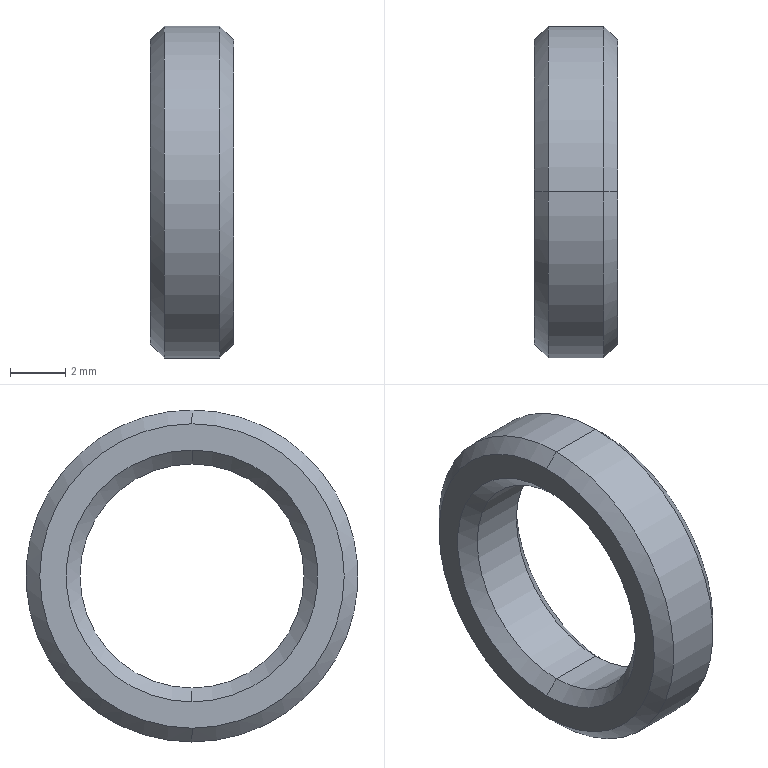Part | STEP file | PN_0017 driven wheel limiting round block_Default | 1 solid | 14 faces | box 3 x 12 x 12 mm | volume 168.916 mm3 | cone 8 | cylinder 4 | plane 2 | commonest cylinder face diameters 8.1 x2 12 x2
STEP:
#1=CARTESIAN_POINT('',(0.,0.,0.));
#2=DIRECTION('',(0.,0.,1.));
#3=DIRECTION('',(1.,0.,0.));
#4=AXIS2_PLACEMENT_3D('',#1,#2,#3);
#5=CARTESIAN_POINT('',(0.5,0.,4.05));
#6=VERTEX_POINT('',#5);
#7=CARTESIAN_POINT('',(0.,0.,4.55));
#8=VERTEX_POINT('',#7);
#9=CARTESIAN_POINT('',(0.,0.,4.55));
#10=DIRECTION('',(-0.7071,0.,0.7071));
#11=VECTOR('',#10,1.);
#12=LINE('',#9,#11);
#13=CARTESIAN_POINT('',(0.,0.,0.));
#14=DIRECTION('',(-1.,0.,0.));
#15=DIRECTION('',(0.,0.,1.));
#16=AXIS2_PLACEMENT_3D('',#13,#14,#15);
#17=CONICAL_SURFACE('',#16,4.55,0.7854);
#18=CARTESIAN_POINT('',(6.283,0.));
#19=DIRECTION('',(0.,1.));
#20=VECTOR('',#19,1.);
#21=LINE('',#18,#20);
#22=(GEOMETRIC_REPRESENTATION_CONTEXT(2)PARAMETRIC_REPRESENTATION_CONTEXT()REPRESENTATION_CONTEXT('',''));
#23=DEFINITIONAL_REPRESENTATION('',(#21),#22);
#24=PCURVE('',#17,#23);
#25=CARTESIAN_POINT('',(0.,0.,0.));
#26=DIRECTION('',(-1.,0.,0.));
#27=DIRECTION('',(0.,0.,1.));
#28=AXIS2_PLACEMENT_3D('',#25,#26,#27);
#29=CONICAL_SURFACE('',#28,4.55,0.7854);
#30=CARTESIAN_POINT('',(0.,0.));
#31=DIRECTION('',(0.,1.));
#32=VECTOR('',#31,1.);
#33=LINE('',#30,#32);
#34=(GEOMETRIC_REPRESENTATION_CONTEXT(2)PARAMETRIC_REPRESENTATION_CONTEXT()REPRESENTATION_CONTEXT('',''));
#35=DEFINITIONAL_REPRESENTATION('',(#33),#34);
#36=PCURVE('',#29,#35);
#37=SURFACE_CURVE('',#12,(#24,#36),.PCURVE_S1.);
#38=EDGE_CURVE('',#6,#8,#37,.T.);
#39=ORIENTED_EDGE('',*,*,#38,.T.);
#40=CARTESIAN_POINT('',(0.,0.,-4.55));
#41=VERTEX_POINT('',#40);
#42=CARTESIAN_POINT('',(0.,0.,0.));
#43=DIRECTION('',(1.,0.,0.));
#44=DIRECTION('',(0.,0.,-1.));
#45=AXIS2_PLACEMENT_3D('',#42,#43,#44);
#46=CIRCLE('',#45,4.55);
#47=CARTESIAN_POINT('',(9.425,0.));
#48=DIRECTION('',(-1.,0.));
#49=VECTOR('',#48,1.);
#50=LINE('',#47,#49);
#51=(GEOMETRIC_REPRESENTATION_CONTEXT(2)PARAMETRIC_REPRESENTATION_CONTEXT()REPRESENTATION_CONTEXT('',''));
#52=DEFINITIONAL_REPRESENTATION('',(#50),#51);
#53=PCURVE('',#17,#52);
#54=CARTESIAN_POINT('',(0.,0.,0.));
#55=DIRECTION('',(1.,0.,0.));
#56=DIRECTION('',(0.,0.,-1.));
#57=AXIS2_PLACEMENT_3D('',#54,#55,#56);
#58=PLANE('',#57);
#59=CARTESIAN_POINT('',(0.,0.));
#60=DIRECTION('',(1.,0.));
#61=AXIS2_PLACEMENT_2D('',#59,#60);
#62=CIRCLE('',#61,4.55);
#63=(GEOMETRIC_REPRESENTATION_CONTEXT(2)PARAMETRIC_REPRESENTATION_CONTEXT()REPRESENTATION_CONTEXT('',''));
#64=DEFINITIONAL_REPRESENTATION('',(#62),#63);
#65=PCURVE('',#58,#64);
#66=SURFACE_CURVE('',#46,(#53,#65),.PCURVE_S1.);
#67=EDGE_CURVE('',#8,#41,#66,.T.);
#68=ORIENTED_EDGE('',*,*,#67,.T.);
#69=CARTESIAN_POINT('',(0.5,0.,-4.05));
#70=VERTEX_POINT('',#69);
#71=CARTESIAN_POINT('',(0.,0.,-4.55));
#72=DIRECTION('',(-0.7071,0.,-0.7071));
#73=VECTOR('',#72,1.);
#74=LINE('',#71,#73);
#75=CARTESIAN_POINT('',(3.142,0.));
#76=DIRECTION('',(0.,1.));
#77=VECTOR('',#76,1.);
#78=LINE('',#75,#77);
#79=(GEOMETRIC_REPRESENTATION_CONTEXT(2)PARAMETRIC_REPRESENTATION_CONTEXT()REPRESENTATION_CONTEXT('',''));
#80=DEFINITIONAL_REPRESENTATION('',(#78),#79);
#81=PCURVE('',#17,#80);
#82=CARTESIAN_POINT('',(3.142,0.));
#83=DIRECTION('',(0.,1.));
#84=VECTOR('',#83,1.);
#85=LINE('',#82,#84);
#86=(GEOMETRIC_REPRESENTATION_CONTEXT(2)PARAMETRIC_REPRESENTATION_CONTEXT()REPRESENTATION_CONTEXT('',''));
#87=DEFINITIONAL_REPRESENTATION('',(#85),#86);
#88=PCURVE('',#29,#87);
#89=SURFACE_CURVE('',#74,(#81,#88),.PCURVE_S1.);
#90=EDGE_CURVE('',#70,#41,#89,.T.);
#91=ORIENTED_EDGE('',*,*,#90,.F.);
#92=CARTESIAN_POINT('',(0.5,0.,0.));
#93=DIRECTION('',(-1.,0.,0.));
#94=DIRECTION('',(0.,0.,-1.));
#95=AXIS2_PLACEMENT_3D('',#92,#93,#94);
#96=CIRCLE('',#95,4.05);
#97=CARTESIAN_POINT('',(3.142,-0.5));
#98=DIRECTION('',(1.,0.));
#99=VECTOR('',#98,1.);
#100=LINE('',#97,#99);
#101=(GEOMETRIC_REPRESENTATION_CONTEXT(2)PARAMETRIC_REPRESENTATION_CONTEXT()REPRESENTATION_CONTEXT('',''));
#102=DEFINITIONAL_REPRESENTATION('',(#100),#101);
#103=PCURVE('',#17,#102);
#104=CARTESIAN_POINT('',(3.,0.,0.));
#105=DIRECTION('',(-1.,0.,0.));
#106=DIRECTION('',(0.,0.,1.));
#107=AXIS2_PLACEMENT_3D('',#104,#105,#106);
#108=CYLINDRICAL_SURFACE('',#107,4.05);
#109=CARTESIAN_POINT('',(3.142,2.5));
#110=DIRECTION('',(1.,0.));
#111=VECTOR('',#110,1.);
#112=LINE('',#109,#111);
#113=(GEOMETRIC_REPRESENTATION_CONTEXT(2)PARAMETRIC_REPRESENTATION_CONTEXT()REPRESENTATION_CONTEXT('',''));
#114=DEFINITIONAL_REPRESENTATION('',(#112),#113);
#115=PCURVE('',#108,#114);
#116=SURFACE_CURVE('',#96,(#103,#115),.PCURVE_S1.);
#117=EDGE_CURVE('',#70,#6,#116,.T.);
#118=ORIENTED_EDGE('',*,*,#117,.T.);
#119=EDGE_LOOP('',(#39,#68,#91,#118));
#120=FACE_BOUND('',#119,.F.);
#121=ADVANCED_FACE('',(#120),#17,.F.);
#122=CARTESIAN_POINT('',(2.5,0.,-4.05));
#123=VERTEX_POINT('',#122);
#124=CARTESIAN_POINT('',(3.,0.,-4.55));
#125=VERTEX_POINT('',#124);
#126=CARTESIAN_POINT('',(2.5,0.,-4.05));
#127=DIRECTION('',(0.7071,0.,-0.7071));
#128=VECTOR('',#127,1.);
#129=LINE('',#126,#128);
#130=CARTESIAN_POINT('',(2.5,0.,0.));
#131=DIRECTION('',(1.,0.,0.));
#132=DIRECTION('',(0.,0.,-1.));
#133=AXIS2_PLACEMENT_3D('',#130,#131,#132);
#134=CONICAL_SURFACE('',#133,4.05,0.7854);
#135=CARTESIAN_POINT('',(6.283,0.));
#136=DIRECTION('',(0.,1.));
#137=VECTOR('',#136,1.);
#138=LINE('',#135,#137);
#139=(GEOMETRIC_REPRESENTATION_CONTEXT(2)PARAMETRIC_REPRESENTATION_CONTEXT()REPRESENTATION_CONTEXT('',''));
#140=DEFINITIONAL_REPRESENTATION('',(#138),#139);
#141=PCURVE('',#134,#140);
#142=CARTESIAN_POINT('',(2.5,0.,0.));
#143=DIRECTION('',(1.,0.,0.));
#144=DIRECTION('',(0.,0.,-1.));
#145=AXIS2_PLACEMENT_3D('',#142,#143,#144);
#146=CONICAL_SURFACE('',#145,4.05,0.7854);
#147=CARTESIAN_POINT('',(0.,0.));
#148=DIRECTION('',(0.,1.));
#149=VECTOR('',#148,1.);
#150=LINE('',#147,#149);
#151=(GEOMETRIC_REPRESENTATION_CONTEXT(2)PARAMETRIC_REPRESENTATION_CONTEXT()REPRESENTATION_CONTEXT('',''));
#152=DEFINITIONAL_REPRESENTATION('',(#150),#151);
#153=PCURVE('',#146,#152);
#154=SURFACE_CURVE('',#129,(#141,#153),.PCURVE_S1.);
#155=EDGE_CURVE('',#123,#125,#154,.T.);
#156=ORIENTED_EDGE('',*,*,#155,.T.);
#157=CARTESIAN_POINT('',(3.,0.,4.55));
#158=VERTEX_POINT('',#157);
#159=CARTESIAN_POINT('',(3.,0.,0.));
#160=DIRECTION('',(-1.,0.,0.));
#161=DIRECTION('',(0.,0.,-1.));
#162=AXIS2_PLACEMENT_3D('',#159,#160,#161);
#163=CIRCLE('',#162,4.55);
#164=CARTESIAN_POINT('',(6.283,0.5));
#165=DIRECTION('',(-1.,0.));
#166=VECTOR('',#165,1.);
#167=LINE('',#164,#166);
#168=(GEOMETRIC_REPRESENTATION_CONTEXT(2)PARAMETRIC_REPRESENTATION_CONTEXT()REPRESENTATION_CONTEXT('',''));
#169=DEFINITIONAL_REPRESENTATION('',(#167),#168);
#170=PCURVE('',#134,#169);
#171=CARTESIAN_POINT('',(3.,0.,0.));
#172=DIRECTION('',(1.,0.,0.));
#173=DIRECTION('',(0.,0.,-1.));
#174=AXIS2_PLACEMENT_3D('',#171,#172,#173);
#175=PLANE('',#174);
#176=CARTESIAN_POINT('',(4.55,0.));
#177=CARTESIAN_POINT('',(4.55,-7.881));
#178=CARTESIAN_POINT('',(-2.275,-3.94));
#179=CARTESIAN_POINT('',(-9.1,0.));
#180=CARTESIAN_POINT('',(-2.275,3.94));
#181=CARTESIAN_POINT('',(4.55,7.881));
#182=CARTESIAN_POINT('',(4.55,0.));
#183=(BOUNDED_CURVE()B_SPLINE_CURVE(2,(#176,#177,#178,#179,#180,#181,#182),.UNSPECIFIED.,.T.,.F.)B_SPLINE_CURVE_WITH_KNOTS((1,2,2,2,2,1),(-2.094,0.,2.094,4.189,6.283,8.378),.UNSPECIFIED.)CURVE()GEOMETRIC_REPRESENTATION_ITEM()RATIONAL_B_SPLINE_CURVE((1.,0.5,1.,0.5,1.,0.5,1.))REPRESENTATION_ITEM(''));
#184=(GEOMETRIC_REPRESENTATION_CONTEXT(2)PARAMETRIC_REPRESENTATION_CONTEXT()REPRESENTATION_CONTEXT('',''));
#185=DEFINITIONAL_REPRESENTATION('',(#183),#184);
#186=PCURVE('',#175,#185);
#187=SURFACE_CURVE('',#163,(#170,#186),.PCURVE_S1.);
#188=EDGE_CURVE('',#125,#158,#187,.T.);
#189=ORIENTED_EDGE('',*,*,#188,.T.);
#190=CARTESIAN_POINT('',(2.5,0.,4.05));
#191=VERTEX_POINT('',#190);
#192=CARTESIAN_POINT('',(2.5,0.,4.05));
#193=DIRECTION('',(0.7071,0.,0.7071));
#194=VECTOR('',#193,1.);
#195=LINE('',#192,#194);
#196=CARTESIAN_POINT('',(3.142,0.));
#197=DIRECTION('',(0.,1.));
#198=VECTOR('',#197,1.);
#199=LINE('',#196,#198);
#200=(GEOMETRIC_REPRESENTATION_CONTEXT(2)PARAMETRIC_REPRESENTATION_CONTEXT()REPRESENTATION_CONTEXT('',''));
#201=DEFINITIONAL_REPRESENTATION('',(#199),#200);
#202=PCURVE('',#134,#201);
#203=CARTESIAN_POINT('',(3.142,0.));
#204=DIRECTION('',(0.,1.));
#205=VECTOR('',#204,1.);
#206=LINE('',#203,#205);
#207=(GEOMETRIC_REPRESENTATION_CONTEXT(2)PARAMETRIC_REPRESENTATION_CONTEXT()REPRESENTATION_CONTEXT('',''));
#208=DEFINITIONAL_REPRESENTATION('',(#206),#207);
#209=PCURVE('',#146,#208);
#210=SURFACE_CURVE('',#195,(#202,#209),.PCURVE_S1.);
#211=EDGE_CURVE('',#191,#158,#210,.T.);
#212=ORIENTED_EDGE('',*,*,#211,.F.);
#213=CARTESIAN_POINT('',(2.5,0.,0.));
#214=DIRECTION('',(1.,0.,0.));
#215=DIRECTION('',(0.,0.,-1.));
#216=AXIS2_PLACEMENT_3D('',#213,#214,#215);
#217=CIRCLE('',#216,4.05);
#218=CARTESIAN_POINT('',(0.,0.));
#219=DIRECTION('',(1.,0.));
#220=VECTOR('',#219,1.);
#221=LINE('',#218,#220);
#222=(GEOMETRIC_REPRESENTATION_CONTEXT(2)PARAMETRIC_REPRESENTATION_CONTEXT()REPRESENTATION_CONTEXT('',''));
#223=DEFINITIONAL_REPRESENTATION('',(#221),#222);
#224=PCURVE('',#134,#223);
#225=CARTESIAN_POINT('',(9.425,0.5));
#226=DIRECTION('',(-1.,0.));
#227=VECTOR('',#226,1.);
#228=LINE('',#225,#227);
#229=(GEOMETRIC_REPRESENTATION_CONTEXT(2)PARAMETRIC_REPRESENTATION_CONTEXT()REPRESENTATION_CONTEXT('',''));
#230=DEFINITIONAL_REPRESENTATION('',(#228),#229);
#231=PCURVE('',#108,#230);
#232=SURFACE_CURVE('',#217,(#224,#231),.PCURVE_S1.);
#233=EDGE_CURVE('',#191,#123,#232,.T.);
#234=ORIENTED_EDGE('',*,*,#233,.T.);
#235=EDGE_LOOP('',(#156,#189,#212,#234));
#236=FACE_BOUND('',#235,.F.);
#237=ADVANCED_FACE('',(#236),#134,.F.);
#238=CARTESIAN_POINT('',(0.,0.,5.5));
#239=VERTEX_POINT('',#238);
#240=CARTESIAN_POINT('',(0.,0.,-5.5));
#241=VERTEX_POINT('',#240);
#242=CARTESIAN_POINT('',(0.,0.,0.));
#243=DIRECTION('',(-1.,0.,0.));
#244=DIRECTION('',(0.,0.,-1.));
#245=AXIS2_PLACEMENT_3D('',#242,#243,#244);
#246=CIRCLE('',#245,5.5);
#247=CARTESIAN_POINT('',(0.5,0.,0.));
#248=DIRECTION('',(1.,0.,0.));
#249=DIRECTION('',(0.,0.,-1.));
#250=AXIS2_PLACEMENT_3D('',#247,#248,#249);
#251=CONICAL_SURFACE('',#250,6.,0.7854);
#252=CARTESIAN_POINT('',(6.283,-0.5));
#253=DIRECTION('',(-1.,0.));
#254=VECTOR('',#253,1.);
#255=LINE('',#252,#254);
#256=(GEOMETRIC_REPRESENTATION_CONTEXT(2)PARAMETRIC_REPRESENTATION_CONTEXT()REPRESENTATION_CONTEXT('',''));
#257=DEFINITIONAL_REPRESENTATION('',(#255),#256);
#258=PCURVE('',#251,#257);
#259=CARTESIAN_POINT('',(5.5,0.));
#260=CARTESIAN_POINT('',(5.5,-9.526));
#261=CARTESIAN_POINT('',(-2.75,-4.763));
#262=CARTESIAN_POINT('',(-11.,0.));
#263=CARTESIAN_POINT('',(-2.75,4.763));
#264=CARTESIAN_POINT('',(5.5,9.526));
#265=CARTESIAN_POINT('',(5.5,0.));
#266=(BOUNDED_CURVE()B_SPLINE_CURVE(2,(#259,#260,#261,#262,#263,#264,#265),.UNSPECIFIED.,.T.,.F.)B_SPLINE_CURVE_WITH_KNOTS((1,2,2,2,2,1),(-2.094,0.,2.094,4.189,6.283,8.378),.UNSPECIFIED.)CURVE()GEOMETRIC_REPRESENTATION_ITEM()RATIONAL_B_SPLINE_CURVE((1.,0.5,1.,0.5,1.,0.5,1.))REPRESENTATION_ITEM(''));
#267=(GEOMETRIC_REPRESENTATION_CONTEXT(2)PARAMETRIC_REPRESENTATION_CONTEXT()REPRESENTATION_CONTEXT('',''));
#268=DEFINITIONAL_REPRESENTATION('',(#266),#267);
#269=PCURVE('',#58,#268);
#270=SURFACE_CURVE('',#246,(#258,#269),.PCURVE_S1.);
#271=EDGE_CURVE('',#239,#241,#270,.T.);
#272=ORIENTED_EDGE('',*,*,#271,.F.);
#273=CARTESIAN_POINT('',(0.5,0.,6.));
#274=VERTEX_POINT('',#273);
#275=CARTESIAN_POINT('',(0.5,0.,6.));
#276=DIRECTION('',(0.7071,0.,0.7071));
#277=VECTOR('',#276,1.);
#278=LINE('',#275,#277);
#279=CARTESIAN_POINT('',(3.142,0.));
#280=DIRECTION('',(0.,1.));
#281=VECTOR('',#280,1.);
#282=LINE('',#279,#281);
#283=(GEOMETRIC_REPRESENTATION_CONTEXT(2)PARAMETRIC_REPRESENTATION_CONTEXT()REPRESENTATION_CONTEXT('',''));
#284=DEFINITIONAL_REPRESENTATION('',(#282),#283);
#285=PCURVE('',#251,#284);
#286=CARTESIAN_POINT('',(0.5,0.,0.));
#287=DIRECTION('',(1.,0.,0.));
#288=DIRECTION('',(0.,0.,-1.));
#289=AXIS2_PLACEMENT_3D('',#286,#287,#288);
#290=CONICAL_SURFACE('',#289,6.,0.7854);
#291=CARTESIAN_POINT('',(3.142,0.));
#292=DIRECTION('',(0.,1.));
#293=VECTOR('',#292,1.);
#294=LINE('',#291,#293);
#295=(GEOMETRIC_REPRESENTATION_CONTEXT(2)PARAMETRIC_REPRESENTATION_CONTEXT()REPRESENTATION_CONTEXT('',''));
#296=DEFINITIONAL_REPRESENTATION('',(#294),#295);
#297=PCURVE('',#290,#296);
#298=SURFACE_CURVE('',#278,(#285,#297),.PCURVE_S1.);
#299=EDGE_CURVE('',#239,#274,#298,.T.);
#300=ORIENTED_EDGE('',*,*,#299,.T.);
#301=CARTESIAN_POINT('',(0.5,0.,-6.));
#302=VERTEX_POINT('',#301);
#303=CARTESIAN_POINT('',(0.5,0.,0.));
#304=DIRECTION('',(1.,0.,0.));
#305=DIRECTION('',(0.,0.,-1.));
#306=AXIS2_PLACEMENT_3D('',#303,#304,#305);
#307=CIRCLE('',#306,6.);
#308=CARTESIAN_POINT('',(0.,0.));
#309=DIRECTION('',(1.,0.));
#310=VECTOR('',#309,1.);
#311=LINE('',#308,#310);
#312=(GEOMETRIC_REPRESENTATION_CONTEXT(2)PARAMETRIC_REPRESENTATION_CONTEXT()REPRESENTATION_CONTEXT('',''));
#313=DEFINITIONAL_REPRESENTATION('',(#311),#312);
#314=PCURVE('',#251,#313);
#315=CARTESIAN_POINT('',(3.,0.,0.));
#316=DIRECTION('',(-1.,0.,0.));
#317=DIRECTION('',(0.,0.,1.));
#318=AXIS2_PLACEMENT_3D('',#315,#316,#317);
#319=CYLINDRICAL_SURFACE('',#318,6.);
#320=CARTESIAN_POINT('',(3.142,2.5));
#321=DIRECTION('',(-1.,0.));
#322=VECTOR('',#321,1.);
#323=LINE('',#320,#322);
#324=(GEOMETRIC_REPRESENTATION_CONTEXT(2)PARAMETRIC_REPRESENTATION_CONTEXT()REPRESENTATION_CONTEXT('',''));
#325=DEFINITIONAL_REPRESENTATION('',(#323),#324);
#326=PCURVE('',#319,#325);
#327=SURFACE_CURVE('',#307,(#314,#326),.PCURVE_S1.);
#328=EDGE_CURVE('',#302,#274,#327,.T.);
#329=ORIENTED_EDGE('',*,*,#328,.F.);
#330=CARTESIAN_POINT('',(0.5,0.,-6.));
#331=DIRECTION('',(0.7071,0.,-0.7071));
#332=VECTOR('',#331,1.);
#333=LINE('',#330,#332);
#334=CARTESIAN_POINT('',(0.,0.));
#335=DIRECTION('',(0.,1.));
#336=VECTOR('',#335,1.);
#337=LINE('',#334,#336);
#338=(GEOMETRIC_REPRESENTATION_CONTEXT(2)PARAMETRIC_REPRESENTATION_CONTEXT()REPRESENTATION_CONTEXT('',''));
#339=DEFINITIONAL_REPRESENTATION('',(#337),#338);
#340=PCURVE('',#251,#339);
#341=CARTESIAN_POINT('',(6.283,0.));
#342=DIRECTION('',(0.,1.));
#343=VECTOR('',#342,1.);
#344=LINE('',#341,#343);
#345=(GEOMETRIC_REPRESENTATION_CONTEXT(2)PARAMETRIC_REPRESENTATION_CONTEXT()REPRESENTATION_CONTEXT('',''));
#346=DEFINITIONAL_REPRESENTATION('',(#344),#345);
#347=PCURVE('',#290,#346);
#348=SURFACE_CURVE('',#333,(#340,#347),.PCURVE_S1.);
#349=EDGE_CURVE('',#241,#302,#348,.T.);
#350=ORIENTED_EDGE('',*,*,#349,.F.);
#351=EDGE_LOOP('',(#272,#300,#329,#350));
#352=FACE_BOUND('',#351,.T.);
#353=ADVANCED_FACE('',(#352),#251,.T.);
#354=CARTESIAN_POINT('',(3.,0.,-5.5));
#355=VERTEX_POINT('',#354);
#356=CARTESIAN_POINT('',(3.,0.,5.5));
#357=VERTEX_POINT('',#356);
#358=CARTESIAN_POINT('',(3.,0.,0.));
#359=DIRECTION('',(1.,0.,0.));
#360=DIRECTION('',(0.,0.,-1.));
#361=AXIS2_PLACEMENT_3D('',#358,#359,#360);
#362=CIRCLE('',#361,5.5);
#363=CARTESIAN_POINT('',(3.,0.,0.));
#364=DIRECTION('',(-1.,0.,0.));
#365=DIRECTION('',(0.,0.,1.));
#366=AXIS2_PLACEMENT_3D('',#363,#364,#365);
#367=CONICAL_SURFACE('',#366,5.5,0.7854);
#368=CARTESIAN_POINT('',(3.142,0.));
#369=DIRECTION('',(-1.,0.));
#370=VECTOR('',#369,1.);
#371=LINE('',#368,#370);
#372=(GEOMETRIC_REPRESENTATION_CONTEXT(2)PARAMETRIC_REPRESENTATION_CONTEXT()REPRESENTATION_CONTEXT('',''));
#373=DEFINITIONAL_REPRESENTATION('',(#371),#372);
#374=PCURVE('',#367,#373);
#375=CARTESIAN_POINT('',(0.,0.));
#376=DIRECTION('',(1.,0.));
#377=AXIS2_PLACEMENT_2D('',#375,#376);
#378=CIRCLE('',#377,5.5);
#379=(GEOMETRIC_REPRESENTATION_CONTEXT(2)PARAMETRIC_REPRESENTATION_CONTEXT()REPRESENTATION_CONTEXT('',''));
#380=DEFINITIONAL_REPRESENTATION('',(#378),#379);
#381=PCURVE('',#175,#380);
#382=SURFACE_CURVE('',#362,(#374,#381),.PCURVE_S1.);
#383=EDGE_CURVE('',#355,#357,#382,.T.);
#384=ORIENTED_EDGE('',*,*,#383,.F.);
#385=CARTESIAN_POINT('',(2.5,0.,-6.));
#386=VERTEX_POINT('',#385);
#387=CARTESIAN_POINT('',(3.,0.,-5.5));
#388=DIRECTION('',(-0.7071,0.,-0.7071));
#389=VECTOR('',#388,1.);
#390=LINE('',#387,#389);
#391=CARTESIAN_POINT('',(3.142,0.));
#392=DIRECTION('',(0.,1.));
#393=VECTOR('',#392,1.);
#394=LINE('',#391,#393);
#395=(GEOMETRIC_REPRESENTATION_CONTEXT(2)PARAMETRIC_REPRESENTATION_CONTEXT()REPRESENTATION_CONTEXT('',''));
#396=DEFINITIONAL_REPRESENTATION('',(#394),#395);
#397=PCURVE('',#367,#396);
#398=CARTESIAN_POINT('',(3.,0.,0.));
#399=DIRECTION('',(-1.,0.,0.));
#400=DIRECTION('',(0.,0.,1.));
#401=AXIS2_PLACEMENT_3D('',#398,#399,#400);
#402=CONICAL_SURFACE('',#401,5.5,0.7854);
#403=CARTESIAN_POINT('',(3.142,0.));
#404=DIRECTION('',(0.,1.));
#405=VECTOR('',#404,1.);
#406=LINE('',#403,#405);
#407=(GEOMETRIC_REPRESENTATION_CONTEXT(2)PARAMETRIC_REPRESENTATION_CONTEXT()REPRESENTATION_CONTEXT('',''));
#408=DEFINITIONAL_REPRESENTATION('',(#406),#407);
#409=PCURVE('',#402,#408);
#410=SURFACE_CURVE('',#390,(#397,#409),.PCURVE_S1.);
#411=EDGE_CURVE('',#355,#386,#410,.T.);
#412=ORIENTED_EDGE('',*,*,#411,.T.);
#413=CARTESIAN_POINT('',(2.5,0.,6.));
#414=VERTEX_POINT('',#413);
#415=CARTESIAN_POINT('',(2.5,0.,0.));
#416=DIRECTION('',(-1.,0.,0.));
#417=DIRECTION('',(0.,0.,-1.));
#418=AXIS2_PLACEMENT_3D('',#415,#416,#417);
#419=CIRCLE('',#418,6.);
#420=CARTESIAN_POINT('',(-3.142,0.5));
#421=DIRECTION('',(1.,0.));
#422=VECTOR('',#421,1.);
#423=LINE('',#420,#422);
#424=(GEOMETRIC_REPRESENTATION_CONTEXT(2)PARAMETRIC_REPRESENTATION_CONTEXT()REPRESENTATION_CONTEXT('',''));
#425=DEFINITIONAL_REPRESENTATION('',(#423),#424);
#426=PCURVE('',#367,#425);
#427=CARTESIAN_POINT('',(-3.142,0.5));
#428=DIRECTION('',(1.,0.));
#429=VECTOR('',#428,1.);
#430=LINE('',#427,#429);
#431=(GEOMETRIC_REPRESENTATION_CONTEXT(2)PARAMETRIC_REPRESENTATION_CONTEXT()REPRESENTATION_CONTEXT('',''));
#432=DEFINITIONAL_REPRESENTATION('',(#430),#431);
#433=PCURVE('',#319,#432);
#434=SURFACE_CURVE('',#419,(#426,#433),.PCURVE_S1.);
#435=EDGE_CURVE('',#414,#386,#434,.T.);
#436=ORIENTED_EDGE('',*,*,#435,.F.);
#437=CARTESIAN_POINT('',(3.,0.,5.5));
#438=DIRECTION('',(-0.7071,0.,0.7071));
#439=VECTOR('',#438,1.);
#440=LINE('',#437,#439);
#441=CARTESIAN_POINT('',(0.,0.));
#442=DIRECTION('',(0.,1.));
#443=VECTOR('',#442,1.);
#444=LINE('',#441,#443);
#445=(GEOMETRIC_REPRESENTATION_CONTEXT(2)PARAMETRIC_REPRESENTATION_CONTEXT()REPRESENTATION_CONTEXT('',''));
#446=DEFINITIONAL_REPRESENTATION('',(#444),#445);
#447=PCURVE('',#367,#446);
#448=CARTESIAN_POINT('',(6.283,0.));
#449=DIRECTION('',(0.,1.));
#450=VECTOR('',#449,1.);
#451=LINE('',#448,#450);
#452=(GEOMETRIC_REPRESENTATION_CONTEXT(2)PARAMETRIC_REPRESENTATION_CONTEXT()REPRESENTATION_CONTEXT('',''));
#453=DEFINITIONAL_REPRESENTATION('',(#451),#452);
#454=PCURVE('',#402,#453);
#455=SURFACE_CURVE('',#440,(#447,#454),.PCURVE_S1.);
#456=EDGE_CURVE('',#357,#414,#455,.T.);
#457=ORIENTED_EDGE('',*,*,#456,.F.);
#458=EDGE_LOOP('',(#384,#412,#436,#457));
#459=FACE_BOUND('',#458,.T.);
#460=ADVANCED_FACE('',(#459),#367,.T.);
#461=CARTESIAN_POINT('',(3.,0.,4.05));
#462=DIRECTION('',(-1.,0.,0.));
#463=VECTOR('',#462,1.);
#464=LINE('',#461,#463);
#465=CARTESIAN_POINT('',(6.283,0.));
#466=DIRECTION('',(0.,1.));
#467=VECTOR('',#466,1.);
#468=LINE('',#465,#467);
#469=(GEOMETRIC_REPRESENTATION_CONTEXT(2)PARAMETRIC_REPRESENTATION_CONTEXT()REPRESENTATION_CONTEXT('',''));
#470=DEFINITIONAL_REPRESENTATION('',(#468),#469);
#471=PCURVE('',#108,#470);
#472=CARTESIAN_POINT('',(3.,0.,0.));
#473=DIRECTION('',(-1.,0.,0.));
#474=DIRECTION('',(0.,0.,1.));
#475=AXIS2_PLACEMENT_3D('',#472,#473,#474);
#476=CYLINDRICAL_SURFACE('',#475,4.05);
#477=CARTESIAN_POINT('',(0.,0.));
#478=DIRECTION('',(0.,1.));
#479=VECTOR('',#478,1.);
#480=LINE('',#477,#479);
#481=(GEOMETRIC_REPRESENTATION_CONTEXT(2)PARAMETRIC_REPRESENTATION_CONTEXT()REPRESENTATION_CONTEXT('',''));
#482=DEFINITIONAL_REPRESENTATION('',(#480),#481);
#483=PCURVE('',#476,#482);
#484=SURFACE_CURVE('',#464,(#471,#483),.PCURVE_S1.);
#485=EDGE_CURVE('',#191,#6,#484,.T.);
#486=ORIENTED_EDGE('',*,*,#485,.T.);
#487=ORIENTED_EDGE('',*,*,#117,.F.);
#488=CARTESIAN_POINT('',(3.,0.,-4.05));
#489=DIRECTION('',(-1.,0.,0.));
#490=VECTOR('',#489,1.);
#491=LINE('',#488,#490);
#492=CARTESIAN_POINT('',(3.142,0.));
#493=DIRECTION('',(0.,1.));
#494=VECTOR('',#493,1.);
#495=LINE('',#492,#494);
#496=(GEOMETRIC_REPRESENTATION_CONTEXT(2)PARAMETRIC_REPRESENTATION_CONTEXT()REPRESENTATION_CONTEXT('',''));
#497=DEFINITIONAL_REPRESENTATION('',(#495),#496);
#498=PCURVE('',#108,#497);
#499=CARTESIAN_POINT('',(3.142,0.));
#500=DIRECTION('',(0.,1.));
#501=VECTOR('',#500,1.);
#502=LINE('',#499,#501);
#503=(GEOMETRIC_REPRESENTATION_CONTEXT(2)PARAMETRIC_REPRESENTATION_CONTEXT()REPRESENTATION_CONTEXT('',''));
#504=DEFINITIONAL_REPRESENTATION('',(#502),#503);
#505=PCURVE('',#476,#504);
#506=SURFACE_CURVE('',#491,(#498,#505),.PCURVE_S1.);
#507=EDGE_CURVE('',#123,#70,#506,.T.);
#508=ORIENTED_EDGE('',*,*,#507,.F.);
#509=ORIENTED_EDGE('',*,*,#233,.F.);
#510=EDGE_LOOP('',(#486,#487,#508,#509));
#511=FACE_BOUND('',#510,.F.);
#512=ADVANCED_FACE('',(#511),#108,.F.);
#513=ORIENTED_EDGE('',*,*,#435,.T.);
#514=CARTESIAN_POINT('',(3.,0.,-6.));
#515=DIRECTION('',(-1.,0.,0.));
#516=VECTOR('',#515,1.);
#517=LINE('',#514,#516);
#518=CARTESIAN_POINT('',(3.142,0.));
#519=DIRECTION('',(0.,1.));
#520=VECTOR('',#519,1.);
#521=LINE('',#518,#520);
#522=(GEOMETRIC_REPRESENTATION_CONTEXT(2)PARAMETRIC_REPRESENTATION_CONTEXT()REPRESENTATION_CONTEXT('',''));
#523=DEFINITIONAL_REPRESENTATION('',(#521),#522);
#524=PCURVE('',#319,#523);
#525=CARTESIAN_POINT('',(3.,0.,0.));
#526=DIRECTION('',(-1.,0.,0.));
#527=DIRECTION('',(0.,0.,1.));
#528=AXIS2_PLACEMENT_3D('',#525,#526,#527);
#529=CYLINDRICAL_SURFACE('',#528,6.);
#530=CARTESIAN_POINT('',(3.142,0.));
#531=DIRECTION('',(0.,1.));
#532=VECTOR('',#531,1.);
#533=LINE('',#530,#532);
#534=(GEOMETRIC_REPRESENTATION_CONTEXT(2)PARAMETRIC_REPRESENTATION_CONTEXT()REPRESENTATION_CONTEXT('',''));
#535=DEFINITIONAL_REPRESENTATION('',(#533),#534);
#536=PCURVE('',#529,#535);
#537=SURFACE_CURVE('',#517,(#524,#536),.PCURVE_S1.);
#538=EDGE_CURVE('',#386,#302,#537,.T.);
#539=ORIENTED_EDGE('',*,*,#538,.T.);
#540=ORIENTED_EDGE('',*,*,#328,.T.);
#541=CARTESIAN_POINT('',(3.,0.,6.));
#542=DIRECTION('',(-1.,0.,0.));
#543=VECTOR('',#542,1.);
#544=LINE('',#541,#543);
#545=CARTESIAN_POINT('',(0.,0.));
#546=DIRECTION('',(0.,1.));
#547=VECTOR('',#546,1.);
#548=LINE('',#545,#547);
#549=(GEOMETRIC_REPRESENTATION_CONTEXT(2)PARAMETRIC_REPRESENTATION_CONTEXT()REPRESENTATION_CONTEXT('',''));
#550=DEFINITIONAL_REPRESENTATION('',(#548),#549);
#551=PCURVE('',#319,#550);
#552=CARTESIAN_POINT('',(6.283,0.));
#553=DIRECTION('',(0.,1.));
#554=VECTOR('',#553,1.);
#555=LINE('',#552,#554);
#556=(GEOMETRIC_REPRESENTATION_CONTEXT(2)PARAMETRIC_REPRESENTATION_CONTEXT()REPRESENTATION_CONTEXT('',''));
#557=DEFINITIONAL_REPRESENTATION('',(#555),#556);
#558=PCURVE('',#529,#557);
#559=SURFACE_CURVE('',#544,(#551,#558),.PCURVE_S1.);
#560=EDGE_CURVE('',#414,#274,#559,.T.);
#561=ORIENTED_EDGE('',*,*,#560,.F.);
#562=EDGE_LOOP('',(#513,#539,#540,#561));
#563=FACE_BOUND('',#562,.T.);
#564=ADVANCED_FACE('',(#563),#319,.T.);
#565=CARTESIAN_POINT('',(3.,0.,0.));
#566=DIRECTION('',(1.,0.,0.));
#567=DIRECTION('',(0.,0.,-1.));
#568=AXIS2_PLACEMENT_3D('',#565,#566,#567);
#569=CIRCLE('',#568,5.5);
#570=CARTESIAN_POINT('',(0.,0.));
#571=DIRECTION('',(1.,0.));
#572=AXIS2_PLACEMENT_2D('',#570,#571);
#573=CIRCLE('',#572,5.5);
#574=(GEOMETRIC_REPRESENTATION_CONTEXT(2)PARAMETRIC_REPRESENTATION_CONTEXT()REPRESENTATION_CONTEXT('',''));
#575=DEFINITIONAL_REPRESENTATION('',(#573),#574);
#576=PCURVE('',#175,#575);
#577=CARTESIAN_POINT('',(9.425,0.));
#578=DIRECTION('',(-1.,0.));
#579=VECTOR('',#578,1.);
#580=LINE('',#577,#579);
#581=(GEOMETRIC_REPRESENTATION_CONTEXT(2)PARAMETRIC_REPRESENTATION_CONTEXT()REPRESENTATION_CONTEXT('',''));
#582=DEFINITIONAL_REPRESENTATION('',(#580),#581);
#583=PCURVE('',#402,#582);
#584=SURFACE_CURVE('',#569,(#576,#583),.PCURVE_S1.);
#585=EDGE_CURVE('',#357,#355,#584,.T.);
#586=ORIENTED_EDGE('',*,*,#585,.T.);
#587=ORIENTED_EDGE('',*,*,#383,.T.);
#588=EDGE_LOOP('',(#586,#587));
#589=FACE_BOUND('',#588,.T.);
#590=ORIENTED_EDGE('',*,*,#188,.T.);
#591=CARTESIAN_POINT('',(3.,0.,0.));
#592=DIRECTION('',(-1.,0.,0.));
#593=DIRECTION('',(0.,0.,-1.));
#594=AXIS2_PLACEMENT_3D('',#591,#592,#593);
#595=CIRCLE('',#594,4.55);
#596=CARTESIAN_POINT('',(4.55,0.));
#597=CARTESIAN_POINT('',(4.55,-7.881));
#598=CARTESIAN_POINT('',(-2.275,-3.94));
#599=CARTESIAN_POINT('',(-9.1,0.));
#600=CARTESIAN_POINT('',(-2.275,3.94));
#601=CARTESIAN_POINT('',(4.55,7.881));
#602=CARTESIAN_POINT('',(4.55,0.));
#603=(BOUNDED_CURVE()B_SPLINE_CURVE(2,(#596,#597,#598,#599,#600,#601,#602),.UNSPECIFIED.,.T.,.F.)B_SPLINE_CURVE_WITH_KNOTS((1,2,2,2,2,1),(-2.094,0.,2.094,4.189,6.283,8.378),.UNSPECIFIED.)CURVE()GEOMETRIC_REPRESENTATION_ITEM()RATIONAL_B_SPLINE_CURVE((1.,0.5,1.,0.5,1.,0.5,1.))REPRESENTATION_ITEM(''));
#604=(GEOMETRIC_REPRESENTATION_CONTEXT(2)PARAMETRIC_REPRESENTATION_CONTEXT()REPRESENTATION_CONTEXT('',''));
#605=DEFINITIONAL_REPRESENTATION('',(#603),#604);
#606=PCURVE('',#175,#605);
#607=CARTESIAN_POINT('',(6.283,0.5));
#608=DIRECTION('',(-1.,0.));
#609=VECTOR('',#608,1.);
#610=LINE('',#607,#609);
#611=(GEOMETRIC_REPRESENTATION_CONTEXT(2)PARAMETRIC_REPRESENTATION_CONTEXT()REPRESENTATION_CONTEXT('',''));
#612=DEFINITIONAL_REPRESENTATION('',(#610),#611);
#613=PCURVE('',#146,#612);
#614=SURFACE_CURVE('',#595,(#606,#613),.PCURVE_S1.);
#615=EDGE_CURVE('',#158,#125,#614,.T.);
#616=ORIENTED_EDGE('',*,*,#615,.T.);
#617=EDGE_LOOP('',(#590,#616));
#618=FACE_BOUND('',#617,.T.);
#619=ADVANCED_FACE('',(#589,#618),#175,.T.);
#620=CARTESIAN_POINT('',(0.,0.,0.));
#621=DIRECTION('',(-1.,0.,0.));
#622=DIRECTION('',(0.,0.,-1.));
#623=AXIS2_PLACEMENT_3D('',#620,#621,#622);
#624=CIRCLE('',#623,5.5);
#625=CARTESIAN_POINT('',(5.5,0.));
#626=CARTESIAN_POINT('',(5.5,-9.526));
#627=CARTESIAN_POINT('',(-2.75,-4.763));
#628=CARTESIAN_POINT('',(-11.,0.));
#629=CARTESIAN_POINT('',(-2.75,4.763));
#630=CARTESIAN_POINT('',(5.5,9.526));
#631=CARTESIAN_POINT('',(5.5,0.));
#632=(BOUNDED_CURVE()B_SPLINE_CURVE(2,(#625,#626,#627,#628,#629,#630,#631),.UNSPECIFIED.,.T.,.F.)B_SPLINE_CURVE_WITH_KNOTS((1,2,2,2,2,1),(-2.094,0.,2.094,4.189,6.283,8.378),.UNSPECIFIED.)CURVE()GEOMETRIC_REPRESENTATION_ITEM()RATIONAL_B_SPLINE_CURVE((1.,0.5,1.,0.5,1.,0.5,1.))REPRESENTATION_ITEM(''));
#633=(GEOMETRIC_REPRESENTATION_CONTEXT(2)PARAMETRIC_REPRESENTATION_CONTEXT()REPRESENTATION_CONTEXT('',''));
#634=DEFINITIONAL_REPRESENTATION('',(#632),#633);
#635=PCURVE('',#58,#634);
#636=CARTESIAN_POINT('',(6.283,-0.5));
#637=DIRECTION('',(-1.,0.));
#638=VECTOR('',#637,1.);
#639=LINE('',#636,#638);
#640=(GEOMETRIC_REPRESENTATION_CONTEXT(2)PARAMETRIC_REPRESENTATION_CONTEXT()REPRESENTATION_CONTEXT('',''));
#641=DEFINITIONAL_REPRESENTATION('',(#639),#640);
#642=PCURVE('',#290,#641);
#643=SURFACE_CURVE('',#624,(#635,#642),.PCURVE_S1.);
#644=EDGE_CURVE('',#241,#239,#643,.T.);
#645=ORIENTED_EDGE('',*,*,#644,.T.);
#646=ORIENTED_EDGE('',*,*,#271,.T.);
#647=EDGE_LOOP('',(#645,#646));
#648=FACE_BOUND('',#647,.T.);
#649=ORIENTED_EDGE('',*,*,#67,.T.);
#650=CARTESIAN_POINT('',(0.,0.,0.));
#651=DIRECTION('',(1.,0.,0.));
#652=DIRECTION('',(0.,0.,-1.));
#653=AXIS2_PLACEMENT_3D('',#650,#651,#652);
#654=CIRCLE('',#653,4.55);
#655=CARTESIAN_POINT('',(0.,0.));
#656=DIRECTION('',(1.,0.));
#657=AXIS2_PLACEMENT_2D('',#655,#656);
#658=CIRCLE('',#657,4.55);
#659=(GEOMETRIC_REPRESENTATION_CONTEXT(2)PARAMETRIC_REPRESENTATION_CONTEXT()REPRESENTATION_CONTEXT('',''));
#660=DEFINITIONAL_REPRESENTATION('',(#658),#659);
#661=PCURVE('',#58,#660);
#662=CARTESIAN_POINT('',(3.142,0.));
#663=DIRECTION('',(-1.,0.));
#664=VECTOR('',#663,1.);
#665=LINE('',#662,#664);
#666=(GEOMETRIC_REPRESENTATION_CONTEXT(2)PARAMETRIC_REPRESENTATION_CONTEXT()REPRESENTATION_CONTEXT('',''));
#667=DEFINITIONAL_REPRESENTATION('',(#665),#666);
#668=PCURVE('',#29,#667);
#669=SURFACE_CURVE('',#654,(#661,#668),.PCURVE_S1.);
#670=EDGE_CURVE('',#41,#8,#669,.T.);
#671=ORIENTED_EDGE('',*,*,#670,.T.);
#672=EDGE_LOOP('',(#649,#671));
#673=FACE_BOUND('',#672,.T.);
#674=ADVANCED_FACE('',(#648,#673),#58,.F.);
#675=ORIENTED_EDGE('',*,*,#538,.F.);
#676=CARTESIAN_POINT('',(2.5,0.,0.));
#677=DIRECTION('',(-1.,0.,0.));
#678=DIRECTION('',(0.,0.,-1.));
#679=AXIS2_PLACEMENT_3D('',#676,#677,#678);
#680=CIRCLE('',#679,6.);
#681=CARTESIAN_POINT('',(3.142,0.5));
#682=DIRECTION('',(1.,0.));
#683=VECTOR('',#682,1.);
#684=LINE('',#681,#683);
#685=(GEOMETRIC_REPRESENTATION_CONTEXT(2)PARAMETRIC_REPRESENTATION_CONTEXT()REPRESENTATION_CONTEXT('',''));
#686=DEFINITIONAL_REPRESENTATION('',(#684),#685);
#687=PCURVE('',#529,#686);
#688=CARTESIAN_POINT('',(3.142,0.5));
#689=DIRECTION('',(1.,0.));
#690=VECTOR('',#689,1.);
#691=LINE('',#688,#690);
#692=(GEOMETRIC_REPRESENTATION_CONTEXT(2)PARAMETRIC_REPRESENTATION_CONTEXT()REPRESENTATION_CONTEXT('',''));
#693=DEFINITIONAL_REPRESENTATION('',(#691),#692);
#694=PCURVE('',#402,#693);
#695=SURFACE_CURVE('',#680,(#687,#694),.PCURVE_S1.);
#696=EDGE_CURVE('',#386,#414,#695,.T.);
#697=ORIENTED_EDGE('',*,*,#696,.T.);
#698=ORIENTED_EDGE('',*,*,#560,.T.);
#699=CARTESIAN_POINT('',(0.5,0.,0.));
#700=DIRECTION('',(1.,0.,0.));
#701=DIRECTION('',(0.,0.,-1.));
#702=AXIS2_PLACEMENT_3D('',#699,#700,#701);
#703=CIRCLE('',#702,6.);
#704=CARTESIAN_POINT('',(9.425,2.5));
#705=DIRECTION('',(-1.,0.));
#706=VECTOR('',#705,1.);
#707=LINE('',#704,#706);
#708=(GEOMETRIC_REPRESENTATION_CONTEXT(2)PARAMETRIC_REPRESENTATION_CONTEXT()REPRESENTATION_CONTEXT('',''));
#709=DEFINITIONAL_REPRESENTATION('',(#707),#708);
#710=PCURVE('',#529,#709);
#711=CARTESIAN_POINT('',(0.,0.));
#712=DIRECTION('',(1.,0.));
#713=VECTOR('',#712,1.);
#714=LINE('',#711,#713);
#715=(GEOMETRIC_REPRESENTATION_CONTEXT(2)PARAMETRIC_REPRESENTATION_CONTEXT()REPRESENTATION_CONTEXT('',''));
#716=DEFINITIONAL_REPRESENTATION('',(#714),#715);
#717=PCURVE('',#290,#716);
#718=SURFACE_CURVE('',#703,(#710,#717),.PCURVE_S1.);
#719=EDGE_CURVE('',#274,#302,#718,.T.);
#720=ORIENTED_EDGE('',*,*,#719,.T.);
#721=EDGE_LOOP('',(#675,#697,#698,#720));
#722=FACE_BOUND('',#721,.T.);
#723=ADVANCED_FACE('',(#722),#529,.T.);
#724=CARTESIAN_POINT('',(0.5,0.,0.));
#725=DIRECTION('',(-1.,0.,0.));
#726=DIRECTION('',(0.,0.,-1.));
#727=AXIS2_PLACEMENT_3D('',#724,#725,#726);
#728=CIRCLE('',#727,4.05);
#729=CARTESIAN_POINT('',(-3.142,2.5));
#730=DIRECTION('',(1.,0.));
#731=VECTOR('',#730,1.);
#732=LINE('',#729,#731);
#733=(GEOMETRIC_REPRESENTATION_CONTEXT(2)PARAMETRIC_REPRESENTATION_CONTEXT()REPRESENTATION_CONTEXT('',''));
#734=DEFINITIONAL_REPRESENTATION('',(#732),#733);
#735=PCURVE('',#476,#734);
#736=CARTESIAN_POINT('',(-3.142,-0.5));
#737=DIRECTION('',(1.,0.));
#738=VECTOR('',#737,1.);
#739=LINE('',#736,#738);
#740=(GEOMETRIC_REPRESENTATION_CONTEXT(2)PARAMETRIC_REPRESENTATION_CONTEXT()REPRESENTATION_CONTEXT('',''));
#741=DEFINITIONAL_REPRESENTATION('',(#739),#740);
#742=PCURVE('',#29,#741);
#743=SURFACE_CURVE('',#728,(#735,#742),.PCURVE_S1.);
#744=EDGE_CURVE('',#6,#70,#743,.T.);
#745=ORIENTED_EDGE('',*,*,#744,.F.);
#746=ORIENTED_EDGE('',*,*,#485,.F.);
#747=CARTESIAN_POINT('',(2.5,0.,0.));
#748=DIRECTION('',(1.,0.,0.));
#749=DIRECTION('',(0.,0.,-1.));
#750=AXIS2_PLACEMENT_3D('',#747,#748,#749);
#751=CIRCLE('',#750,4.05);
#752=CARTESIAN_POINT('',(3.142,0.5));
#753=DIRECTION('',(-1.,0.));
#754=VECTOR('',#753,1.);
#755=LINE('',#752,#754);
#756=(GEOMETRIC_REPRESENTATION_CONTEXT(2)PARAMETRIC_REPRESENTATION_CONTEXT()REPRESENTATION_CONTEXT('',''));
#757=DEFINITIONAL_REPRESENTATION('',(#755),#756);
#758=PCURVE('',#476,#757);
#759=CARTESIAN_POINT('',(0.,0.));
#760=DIRECTION('',(1.,0.));
#761=VECTOR('',#760,1.);
#762=LINE('',#759,#761);
#763=(GEOMETRIC_REPRESENTATION_CONTEXT(2)PARAMETRIC_REPRESENTATION_CONTEXT()REPRESENTATION_CONTEXT('',''));
#764=DEFINITIONAL_REPRESENTATION('',(#762),#763);
#765=PCURVE('',#146,#764);
#766=SURFACE_CURVE('',#751,(#758,#765),.PCURVE_S1.);
#767=EDGE_CURVE('',#123,#191,#766,.T.);
#768=ORIENTED_EDGE('',*,*,#767,.F.);
#769=ORIENTED_EDGE('',*,*,#507,.T.);
#770=EDGE_LOOP('',(#745,#746,#768,#769));
#771=FACE_BOUND('',#770,.F.);
#772=ADVANCED_FACE('',(#771),#476,.F.);
#773=ORIENTED_EDGE('',*,*,#411,.F.);
#774=ORIENTED_EDGE('',*,*,#585,.F.);
#775=ORIENTED_EDGE('',*,*,#456,.T.);
#776=ORIENTED_EDGE('',*,*,#696,.F.);
#777=EDGE_LOOP('',(#773,#774,#775,#776));
#778=FACE_BOUND('',#777,.T.);
#779=ADVANCED_FACE('',(#778),#402,.T.);
#780=ORIENTED_EDGE('',*,*,#299,.F.);
#781=ORIENTED_EDGE('',*,*,#644,.F.);
#782=ORIENTED_EDGE('',*,*,#349,.T.);
#783=ORIENTED_EDGE('',*,*,#719,.F.);
#784=EDGE_LOOP('',(#780,#781,#782,#783));
#785=FACE_BOUND('',#784,.T.);
#786=ADVANCED_FACE('',(#785),#290,.T.);
#787=ORIENTED_EDGE('',*,*,#615,.T.);
#788=ORIENTED_EDGE('',*,*,#155,.F.);
#789=ORIENTED_EDGE('',*,*,#767,.T.);
#790=ORIENTED_EDGE('',*,*,#211,.T.);
#791=EDGE_LOOP('',(#787,#788,#789,#790));
#792=FACE_BOUND('',#791,.F.);
#793=ADVANCED_FACE('',(#792),#146,.F.);
#794=ORIENTED_EDGE('',*,*,#670,.T.);
#795=ORIENTED_EDGE('',*,*,#38,.F.);
#796=ORIENTED_EDGE('',*,*,#744,.T.);
#797=ORIENTED_EDGE('',*,*,#90,.T.);
#798=EDGE_LOOP('',(#794,#795,#796,#797));
#799=FACE_BOUND('',#798,.F.);
#800=ADVANCED_FACE('',(#799),#29,.F.);
#801=CLOSED_SHELL('',(#121,#237,#353,#460,#512,#564,#619,#674,#723,#772,#779,#786,#793,#800));
#802=MANIFOLD_SOLID_BREP('',#801);
#803=(LENGTH_UNIT()NAMED_UNIT(*)SI_UNIT(.MILLI.,.METRE.));
#804=UNCERTAINTY_MEASURE_WITH_UNIT(LENGTH_MEASURE(0.0000001),#803,'','');
#805=(NAMED_UNIT(*)PLANE_ANGLE_UNIT()SI_UNIT($,.RADIAN.));
#806=(NAMED_UNIT(*)SI_UNIT($,.STERADIAN.)SOLID_ANGLE_UNIT());
#807=(GEOMETRIC_REPRESENTATION_CONTEXT(3)GLOBAL_UNCERTAINTY_ASSIGNED_CONTEXT((#804))GLOBAL_UNIT_ASSIGNED_CONTEXT((#803,#805,#806))REPRESENTATION_CONTEXT('',''));
#808=ADVANCED_BREP_SHAPE_REPRESENTATION('',(#4,#802),#807);